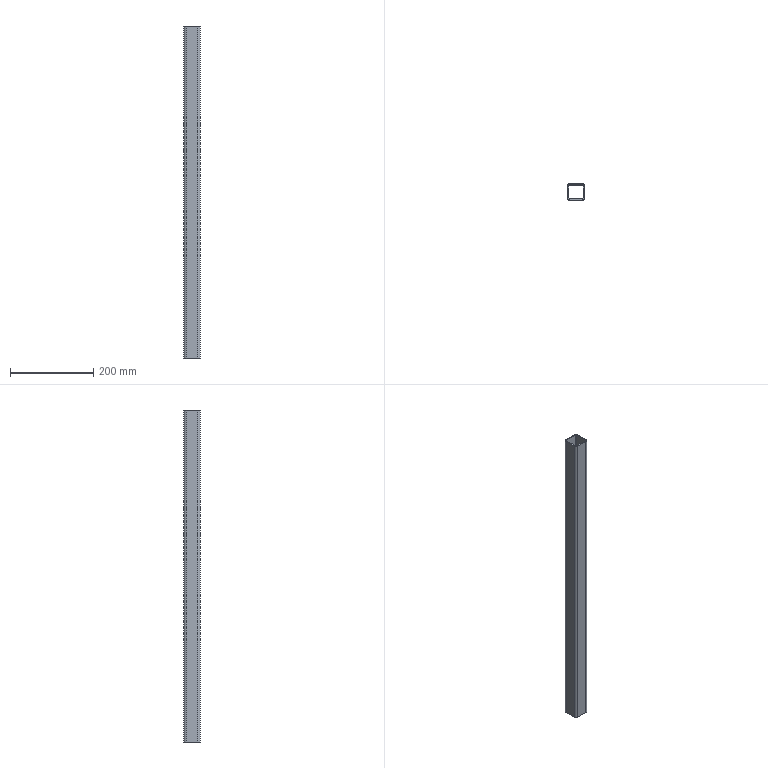Part | STEP file | SN10_002_008-03_TUBO_QUADRADO | 1 solid | 18 faces | box 40 x 40 x 800 mm | volume 336658 mm3 | plane 10 | cylinder 8 | commonest cylinder face diameters 6 x4 12 x4
STEP:
#1=CARTESIAN_POINT('',(0.,0.,0.));
#2=DIRECTION('',(0.,0.,1.));
#3=DIRECTION('',(1.,0.,0.));
#4=AXIS2_PLACEMENT_3D('',#1,#2,#3);
#5=CARTESIAN_POINT('',(20.,14.,-800.));
#6=VERTEX_POINT('',#5);
#7=CARTESIAN_POINT('',(14.,20.,-800.));
#8=VERTEX_POINT('',#7);
#9=CARTESIAN_POINT('',(14.,14.,-800.));
#10=DIRECTION('',(0.,0.,1.));
#11=DIRECTION('',(1.,0.,0.));
#12=AXIS2_PLACEMENT_3D('',#9,#10,#11);
#13=CIRCLE('',#12,6.);
#14=CARTESIAN_POINT('',(14.,14.,-400.));
#15=DIRECTION('',(0.,0.,1.));
#16=DIRECTION('',(1.,0.,0.));
#17=AXIS2_PLACEMENT_3D('',#14,#15,#16);
#18=CYLINDRICAL_SURFACE('',#17,6.);
#19=CARTESIAN_POINT('',(0.,-400.));
#20=DIRECTION('',(1.,0.));
#21=VECTOR('',#20,1.);
#22=LINE('',#19,#21);
#23=(GEOMETRIC_REPRESENTATION_CONTEXT(2)PARAMETRIC_REPRESENTATION_CONTEXT()REPRESENTATION_CONTEXT('',''));
#24=DEFINITIONAL_REPRESENTATION('',(#22),#23);
#25=PCURVE('',#18,#24);
#26=CARTESIAN_POINT('',(0.,0.,-800.));
#27=DIRECTION('',(0.,0.,1.));
#28=DIRECTION('',(1.,0.,0.));
#29=AXIS2_PLACEMENT_3D('',#26,#27,#28);
#30=PLANE('',#29);
#31=CARTESIAN_POINT('',(14.,14.));
#32=DIRECTION('',(1.,0.));
#33=AXIS2_PLACEMENT_2D('',#31,#32);
#34=CIRCLE('',#33,6.);
#35=(GEOMETRIC_REPRESENTATION_CONTEXT(2)PARAMETRIC_REPRESENTATION_CONTEXT()REPRESENTATION_CONTEXT('',''));
#36=DEFINITIONAL_REPRESENTATION('',(#34),#35);
#37=PCURVE('',#30,#36);
#38=SURFACE_CURVE('',#13,(#25,#37),.PCURVE_S1.);
#39=EDGE_CURVE('',#6,#8,#38,.T.);
#40=ORIENTED_EDGE('',*,*,#39,.T.);
#41=CARTESIAN_POINT('',(14.,20.,0.));
#42=VERTEX_POINT('',#41);
#43=CARTESIAN_POINT('',(14.,20.,-800.));
#44=DIRECTION('',(0.,0.,1.));
#45=VECTOR('',#44,1.);
#46=LINE('',#43,#45);
#47=CARTESIAN_POINT('',(1.571,-400.));
#48=DIRECTION('',(0.,1.));
#49=VECTOR('',#48,1.);
#50=LINE('',#47,#49);
#51=(GEOMETRIC_REPRESENTATION_CONTEXT(2)PARAMETRIC_REPRESENTATION_CONTEXT()REPRESENTATION_CONTEXT('',''));
#52=DEFINITIONAL_REPRESENTATION('',(#50),#51);
#53=PCURVE('',#18,#52);
#54=CARTESIAN_POINT('',(-14.,20.,0.));
#55=DIRECTION('',(0.,1.,0.));
#56=DIRECTION('',(0.,0.,1.));
#57=AXIS2_PLACEMENT_3D('',#54,#55,#56);
#58=PLANE('',#57);
#59=CARTESIAN_POINT('',(-800.,28.));
#60=DIRECTION('',(1.,0.));
#61=VECTOR('',#60,1.);
#62=LINE('',#59,#61);
#63=(GEOMETRIC_REPRESENTATION_CONTEXT(2)PARAMETRIC_REPRESENTATION_CONTEXT()REPRESENTATION_CONTEXT('',''));
#64=DEFINITIONAL_REPRESENTATION('',(#62),#63);
#65=PCURVE('',#58,#64);
#66=SURFACE_CURVE('',#46,(#53,#65),.PCURVE_S1.);
#67=EDGE_CURVE('',#8,#42,#66,.T.);
#68=ORIENTED_EDGE('',*,*,#67,.T.);
#69=CARTESIAN_POINT('',(20.,14.,0.));
#70=VERTEX_POINT('',#69);
#71=CARTESIAN_POINT('',(14.,14.,0.));
#72=DIRECTION('',(0.,0.,1.));
#73=DIRECTION('',(1.,0.,0.));
#74=AXIS2_PLACEMENT_3D('',#71,#72,#73);
#75=CIRCLE('',#74,6.);
#76=CARTESIAN_POINT('',(0.,400.));
#77=DIRECTION('',(1.,0.));
#78=VECTOR('',#77,1.);
#79=LINE('',#76,#78);
#80=(GEOMETRIC_REPRESENTATION_CONTEXT(2)PARAMETRIC_REPRESENTATION_CONTEXT()REPRESENTATION_CONTEXT('',''));
#81=DEFINITIONAL_REPRESENTATION('',(#79),#80);
#82=PCURVE('',#18,#81);
#83=CARTESIAN_POINT('',(0.,0.,0.));
#84=DIRECTION('',(0.,0.,1.));
#85=DIRECTION('',(1.,0.,0.));
#86=AXIS2_PLACEMENT_3D('',#83,#84,#85);
#87=PLANE('',#86);
#88=CARTESIAN_POINT('',(14.,14.));
#89=DIRECTION('',(1.,0.));
#90=AXIS2_PLACEMENT_2D('',#88,#89);
#91=CIRCLE('',#90,6.);
#92=(GEOMETRIC_REPRESENTATION_CONTEXT(2)PARAMETRIC_REPRESENTATION_CONTEXT()REPRESENTATION_CONTEXT('',''));
#93=DEFINITIONAL_REPRESENTATION('',(#91),#92);
#94=PCURVE('',#87,#93);
#95=SURFACE_CURVE('',#75,(#82,#94),.PCURVE_S1.);
#96=EDGE_CURVE('',#70,#42,#95,.T.);
#97=ORIENTED_EDGE('',*,*,#96,.F.);
#98=CARTESIAN_POINT('',(20.,14.,-800.));
#99=DIRECTION('',(0.,0.,1.));
#100=VECTOR('',#99,1.);
#101=LINE('',#98,#100);
#102=CARTESIAN_POINT('',(0.,-400.));
#103=DIRECTION('',(0.,1.));
#104=VECTOR('',#103,1.);
#105=LINE('',#102,#104);
#106=(GEOMETRIC_REPRESENTATION_CONTEXT(2)PARAMETRIC_REPRESENTATION_CONTEXT()REPRESENTATION_CONTEXT('',''));
#107=DEFINITIONAL_REPRESENTATION('',(#105),#106);
#108=PCURVE('',#18,#107);
#109=CARTESIAN_POINT('',(20.,14.,0.));
#110=DIRECTION('',(1.,0.,0.));
#111=DIRECTION('',(0.,0.,-1.));
#112=AXIS2_PLACEMENT_3D('',#109,#110,#111);
#113=PLANE('',#112);
#114=CARTESIAN_POINT('',(800.,0.));
#115=DIRECTION('',(-1.,0.));
#116=VECTOR('',#115,1.);
#117=LINE('',#114,#116);
#118=(GEOMETRIC_REPRESENTATION_CONTEXT(2)PARAMETRIC_REPRESENTATION_CONTEXT()REPRESENTATION_CONTEXT('',''));
#119=DEFINITIONAL_REPRESENTATION('',(#117),#118);
#120=PCURVE('',#113,#119);
#121=SURFACE_CURVE('',#101,(#108,#120),.PCURVE_S1.);
#122=EDGE_CURVE('',#6,#70,#121,.T.);
#123=ORIENTED_EDGE('',*,*,#122,.F.);
#124=EDGE_LOOP('',(#40,#68,#97,#123));
#125=FACE_BOUND('',#124,.T.);
#126=ADVANCED_FACE('',(#125),#18,.T.);
#127=CARTESIAN_POINT('',(-14.,20.,-800.));
#128=VERTEX_POINT('',#127);
#129=CARTESIAN_POINT('',(-14.,20.,-800.));
#130=DIRECTION('',(1.,0.,0.));
#131=VECTOR('',#130,1.);
#132=LINE('',#129,#131);
#133=CARTESIAN_POINT('',(-800.,0.));
#134=DIRECTION('',(0.,1.));
#135=VECTOR('',#134,1.);
#136=LINE('',#133,#135);
#137=(GEOMETRIC_REPRESENTATION_CONTEXT(2)PARAMETRIC_REPRESENTATION_CONTEXT()REPRESENTATION_CONTEXT('',''));
#138=DEFINITIONAL_REPRESENTATION('',(#136),#137);
#139=PCURVE('',#58,#138);
#140=CARTESIAN_POINT('',(-14.,20.));
#141=DIRECTION('',(1.,0.));
#142=VECTOR('',#141,1.);
#143=LINE('',#140,#142);
#144=(GEOMETRIC_REPRESENTATION_CONTEXT(2)PARAMETRIC_REPRESENTATION_CONTEXT()REPRESENTATION_CONTEXT('',''));
#145=DEFINITIONAL_REPRESENTATION('',(#143),#144);
#146=PCURVE('',#30,#145);
#147=SURFACE_CURVE('',#132,(#139,#146),.PCURVE_S1.);
#148=EDGE_CURVE('',#128,#8,#147,.T.);
#149=ORIENTED_EDGE('',*,*,#148,.F.);
#150=CARTESIAN_POINT('',(-14.,20.,0.));
#151=VERTEX_POINT('',#150);
#152=CARTESIAN_POINT('',(-14.,20.,0.));
#153=DIRECTION('',(0.,0.,-1.));
#154=VECTOR('',#153,1.);
#155=LINE('',#152,#154);
#156=CARTESIAN_POINT('',(0.,0.));
#157=DIRECTION('',(-1.,0.));
#158=VECTOR('',#157,1.);
#159=LINE('',#156,#158);
#160=(GEOMETRIC_REPRESENTATION_CONTEXT(2)PARAMETRIC_REPRESENTATION_CONTEXT()REPRESENTATION_CONTEXT('',''));
#161=DEFINITIONAL_REPRESENTATION('',(#159),#160);
#162=PCURVE('',#58,#161);
#163=CARTESIAN_POINT('',(-14.,14.,-400.));
#164=DIRECTION('',(0.,0.,1.));
#165=DIRECTION('',(0.,1.,0.));
#166=AXIS2_PLACEMENT_3D('',#163,#164,#165);
#167=CYLINDRICAL_SURFACE('',#166,6.);
#168=CARTESIAN_POINT('',(0.,400.));
#169=DIRECTION('',(0.,-1.));
#170=VECTOR('',#169,1.);
#171=LINE('',#168,#170);
#172=(GEOMETRIC_REPRESENTATION_CONTEXT(2)PARAMETRIC_REPRESENTATION_CONTEXT()REPRESENTATION_CONTEXT('',''));
#173=DEFINITIONAL_REPRESENTATION('',(#171),#172);
#174=PCURVE('',#167,#173);
#175=SURFACE_CURVE('',#155,(#162,#174),.PCURVE_S1.);
#176=EDGE_CURVE('',#151,#128,#175,.T.);
#177=ORIENTED_EDGE('',*,*,#176,.F.);
#178=CARTESIAN_POINT('',(-14.,20.,0.));
#179=DIRECTION('',(1.,0.,0.));
#180=VECTOR('',#179,1.);
#181=LINE('',#178,#180);
#182=CARTESIAN_POINT('',(0.,0.));
#183=DIRECTION('',(0.,1.));
#184=VECTOR('',#183,1.);
#185=LINE('',#182,#184);
#186=(GEOMETRIC_REPRESENTATION_CONTEXT(2)PARAMETRIC_REPRESENTATION_CONTEXT()REPRESENTATION_CONTEXT('',''));
#187=DEFINITIONAL_REPRESENTATION('',(#185),#186);
#188=PCURVE('',#58,#187);
#189=CARTESIAN_POINT('',(-14.,20.));
#190=DIRECTION('',(1.,0.));
#191=VECTOR('',#190,1.);
#192=LINE('',#189,#191);
#193=(GEOMETRIC_REPRESENTATION_CONTEXT(2)PARAMETRIC_REPRESENTATION_CONTEXT()REPRESENTATION_CONTEXT('',''));
#194=DEFINITIONAL_REPRESENTATION('',(#192),#193);
#195=PCURVE('',#87,#194);
#196=SURFACE_CURVE('',#181,(#188,#195),.PCURVE_S1.);
#197=EDGE_CURVE('',#151,#42,#196,.T.);
#198=ORIENTED_EDGE('',*,*,#197,.T.);
#199=ORIENTED_EDGE('',*,*,#67,.F.);
#200=EDGE_LOOP('',(#149,#177,#198,#199));
#201=FACE_BOUND('',#200,.T.);
#202=ADVANCED_FACE('',(#201),#58,.T.);
#203=CARTESIAN_POINT('',(-20.,14.,-800.));
#204=VERTEX_POINT('',#203);
#205=CARTESIAN_POINT('',(-14.,14.,-800.));
#206=DIRECTION('',(0.,0.,1.));
#207=DIRECTION('',(1.,0.,0.));
#208=AXIS2_PLACEMENT_3D('',#205,#206,#207);
#209=CIRCLE('',#208,6.);
#210=CARTESIAN_POINT('',(-1.571,-400.));
#211=DIRECTION('',(1.,0.));
#212=VECTOR('',#211,1.);
#213=LINE('',#210,#212);
#214=(GEOMETRIC_REPRESENTATION_CONTEXT(2)PARAMETRIC_REPRESENTATION_CONTEXT()REPRESENTATION_CONTEXT('',''));
#215=DEFINITIONAL_REPRESENTATION('',(#213),#214);
#216=PCURVE('',#167,#215);
#217=CARTESIAN_POINT('',(-14.,14.));
#218=DIRECTION('',(1.,0.));
#219=AXIS2_PLACEMENT_2D('',#217,#218);
#220=CIRCLE('',#219,6.);
#221=(GEOMETRIC_REPRESENTATION_CONTEXT(2)PARAMETRIC_REPRESENTATION_CONTEXT()REPRESENTATION_CONTEXT('',''));
#222=DEFINITIONAL_REPRESENTATION('',(#220),#221);
#223=PCURVE('',#30,#222);
#224=SURFACE_CURVE('',#209,(#216,#223),.PCURVE_S1.);
#225=EDGE_CURVE('',#128,#204,#224,.T.);
#226=ORIENTED_EDGE('',*,*,#225,.T.);
#227=CARTESIAN_POINT('',(-20.,14.,0.));
#228=VERTEX_POINT('',#227);
#229=CARTESIAN_POINT('',(-20.,14.,-800.));
#230=DIRECTION('',(0.,0.,1.));
#231=VECTOR('',#230,1.);
#232=LINE('',#229,#231);
#233=CARTESIAN_POINT('',(1.571,-400.));
#234=DIRECTION('',(0.,1.));
#235=VECTOR('',#234,1.);
#236=LINE('',#233,#235);
#237=(GEOMETRIC_REPRESENTATION_CONTEXT(2)PARAMETRIC_REPRESENTATION_CONTEXT()REPRESENTATION_CONTEXT('',''));
#238=DEFINITIONAL_REPRESENTATION('',(#236),#237);
#239=PCURVE('',#167,#238);
#240=CARTESIAN_POINT('',(-20.,-14.,0.));
#241=DIRECTION('',(-1.,0.,0.));
#242=DIRECTION('',(0.,0.,1.));
#243=AXIS2_PLACEMENT_3D('',#240,#241,#242);
#244=PLANE('',#243);
#245=CARTESIAN_POINT('',(-800.,28.));
#246=DIRECTION('',(1.,0.));
#247=VECTOR('',#246,1.);
#248=LINE('',#245,#247);
#249=(GEOMETRIC_REPRESENTATION_CONTEXT(2)PARAMETRIC_REPRESENTATION_CONTEXT()REPRESENTATION_CONTEXT('',''));
#250=DEFINITIONAL_REPRESENTATION('',(#248),#249);
#251=PCURVE('',#244,#250);
#252=SURFACE_CURVE('',#232,(#239,#251),.PCURVE_S1.);
#253=EDGE_CURVE('',#204,#228,#252,.T.);
#254=ORIENTED_EDGE('',*,*,#253,.T.);
#255=CARTESIAN_POINT('',(-14.,14.,0.));
#256=DIRECTION('',(0.,0.,1.));
#257=DIRECTION('',(1.,0.,0.));
#258=AXIS2_PLACEMENT_3D('',#255,#256,#257);
#259=CIRCLE('',#258,6.);
#260=CARTESIAN_POINT('',(-1.571,400.));
#261=DIRECTION('',(1.,0.));
#262=VECTOR('',#261,1.);
#263=LINE('',#260,#262);
#264=(GEOMETRIC_REPRESENTATION_CONTEXT(2)PARAMETRIC_REPRESENTATION_CONTEXT()REPRESENTATION_CONTEXT('',''));
#265=DEFINITIONAL_REPRESENTATION('',(#263),#264);
#266=PCURVE('',#167,#265);
#267=CARTESIAN_POINT('',(-14.,14.));
#268=DIRECTION('',(1.,0.));
#269=AXIS2_PLACEMENT_2D('',#267,#268);
#270=CIRCLE('',#269,6.);
#271=(GEOMETRIC_REPRESENTATION_CONTEXT(2)PARAMETRIC_REPRESENTATION_CONTEXT()REPRESENTATION_CONTEXT('',''));
#272=DEFINITIONAL_REPRESENTATION('',(#270),#271);
#273=PCURVE('',#87,#272);
#274=SURFACE_CURVE('',#259,(#266,#273),.PCURVE_S1.);
#275=EDGE_CURVE('',#151,#228,#274,.T.);
#276=ORIENTED_EDGE('',*,*,#275,.F.);
#277=ORIENTED_EDGE('',*,*,#176,.T.);
#278=EDGE_LOOP('',(#226,#254,#276,#277));
#279=FACE_BOUND('',#278,.T.);
#280=ADVANCED_FACE('',(#279),#167,.T.);
#281=CARTESIAN_POINT('',(-20.,-14.,-800.));
#282=VERTEX_POINT('',#281);
#283=CARTESIAN_POINT('',(-20.,-14.,-800.));
#284=DIRECTION('',(0.,1.,0.));
#285=VECTOR('',#284,1.);
#286=LINE('',#283,#285);
#287=CARTESIAN_POINT('',(-800.,0.));
#288=DIRECTION('',(0.,1.));
#289=VECTOR('',#288,1.);
#290=LINE('',#287,#289);
#291=(GEOMETRIC_REPRESENTATION_CONTEXT(2)PARAMETRIC_REPRESENTATION_CONTEXT()REPRESENTATION_CONTEXT('',''));
#292=DEFINITIONAL_REPRESENTATION('',(#290),#291);
#293=PCURVE('',#244,#292);
#294=CARTESIAN_POINT('',(-20.,-14.));
#295=DIRECTION('',(0.,1.));
#296=VECTOR('',#295,1.);
#297=LINE('',#294,#296);
#298=(GEOMETRIC_REPRESENTATION_CONTEXT(2)PARAMETRIC_REPRESENTATION_CONTEXT()REPRESENTATION_CONTEXT('',''));
#299=DEFINITIONAL_REPRESENTATION('',(#297),#298);
#300=PCURVE('',#30,#299);
#301=SURFACE_CURVE('',#286,(#293,#300),.PCURVE_S1.);
#302=EDGE_CURVE('',#282,#204,#301,.T.);
#303=ORIENTED_EDGE('',*,*,#302,.F.);
#304=CARTESIAN_POINT('',(-20.,-14.,0.));
#305=VERTEX_POINT('',#304);
#306=CARTESIAN_POINT('',(-20.,-14.,0.));
#307=DIRECTION('',(0.,0.,-1.));
#308=VECTOR('',#307,1.);
#309=LINE('',#306,#308);
#310=CARTESIAN_POINT('',(0.,0.));
#311=DIRECTION('',(-1.,0.));
#312=VECTOR('',#311,1.);
#313=LINE('',#310,#312);
#314=(GEOMETRIC_REPRESENTATION_CONTEXT(2)PARAMETRIC_REPRESENTATION_CONTEXT()REPRESENTATION_CONTEXT('',''));
#315=DEFINITIONAL_REPRESENTATION('',(#313),#314);
#316=PCURVE('',#244,#315);
#317=CARTESIAN_POINT('',(-14.,-14.,-400.));
#318=DIRECTION('',(0.,0.,1.));
#319=DIRECTION('',(-1.,0.,0.));
#320=AXIS2_PLACEMENT_3D('',#317,#318,#319);
#321=CYLINDRICAL_SURFACE('',#320,6.);
#322=CARTESIAN_POINT('',(0.,400.));
#323=DIRECTION('',(0.,-1.));
#324=VECTOR('',#323,1.);
#325=LINE('',#322,#324);
#326=(GEOMETRIC_REPRESENTATION_CONTEXT(2)PARAMETRIC_REPRESENTATION_CONTEXT()REPRESENTATION_CONTEXT('',''));
#327=DEFINITIONAL_REPRESENTATION('',(#325),#326);
#328=PCURVE('',#321,#327);
#329=SURFACE_CURVE('',#309,(#316,#328),.PCURVE_S1.);
#330=EDGE_CURVE('',#305,#282,#329,.T.);
#331=ORIENTED_EDGE('',*,*,#330,.F.);
#332=CARTESIAN_POINT('',(-20.,-14.,0.));
#333=DIRECTION('',(0.,1.,0.));
#334=VECTOR('',#333,1.);
#335=LINE('',#332,#334);
#336=CARTESIAN_POINT('',(0.,0.));
#337=DIRECTION('',(0.,1.));
#338=VECTOR('',#337,1.);
#339=LINE('',#336,#338);
#340=(GEOMETRIC_REPRESENTATION_CONTEXT(2)PARAMETRIC_REPRESENTATION_CONTEXT()REPRESENTATION_CONTEXT('',''));
#341=DEFINITIONAL_REPRESENTATION('',(#339),#340);
#342=PCURVE('',#244,#341);
#343=CARTESIAN_POINT('',(-20.,-14.));
#344=DIRECTION('',(0.,1.));
#345=VECTOR('',#344,1.);
#346=LINE('',#343,#345);
#347=(GEOMETRIC_REPRESENTATION_CONTEXT(2)PARAMETRIC_REPRESENTATION_CONTEXT()REPRESENTATION_CONTEXT('',''));
#348=DEFINITIONAL_REPRESENTATION('',(#346),#347);
#349=PCURVE('',#87,#348);
#350=SURFACE_CURVE('',#335,(#342,#349),.PCURVE_S1.);
#351=EDGE_CURVE('',#305,#228,#350,.T.);
#352=ORIENTED_EDGE('',*,*,#351,.T.);
#353=ORIENTED_EDGE('',*,*,#253,.F.);
#354=EDGE_LOOP('',(#303,#331,#352,#353));
#355=FACE_BOUND('',#354,.T.);
#356=ADVANCED_FACE('',(#355),#244,.T.);
#357=CARTESIAN_POINT('',(-14.,-20.,-800.));
#358=VERTEX_POINT('',#357);
#359=CARTESIAN_POINT('',(-14.,-14.,-800.));
#360=DIRECTION('',(0.,0.,1.));
#361=DIRECTION('',(1.,0.,0.));
#362=AXIS2_PLACEMENT_3D('',#359,#360,#361);
#363=CIRCLE('',#362,6.);
#364=CARTESIAN_POINT('',(-3.142,-400.));
#365=DIRECTION('',(1.,0.));
#366=VECTOR('',#365,1.);
#367=LINE('',#364,#366);
#368=(GEOMETRIC_REPRESENTATION_CONTEXT(2)PARAMETRIC_REPRESENTATION_CONTEXT()REPRESENTATION_CONTEXT('',''));
#369=DEFINITIONAL_REPRESENTATION('',(#367),#368);
#370=PCURVE('',#321,#369);
#371=CARTESIAN_POINT('',(-14.,-14.));
#372=DIRECTION('',(1.,0.));
#373=AXIS2_PLACEMENT_2D('',#371,#372);
#374=CIRCLE('',#373,6.);
#375=(GEOMETRIC_REPRESENTATION_CONTEXT(2)PARAMETRIC_REPRESENTATION_CONTEXT()REPRESENTATION_CONTEXT('',''));
#376=DEFINITIONAL_REPRESENTATION('',(#374),#375);
#377=PCURVE('',#30,#376);
#378=SURFACE_CURVE('',#363,(#370,#377),.PCURVE_S1.);
#379=EDGE_CURVE('',#282,#358,#378,.T.);
#380=ORIENTED_EDGE('',*,*,#379,.T.);
#381=CARTESIAN_POINT('',(-14.,-20.,0.));
#382=VERTEX_POINT('',#381);
#383=CARTESIAN_POINT('',(-14.,-20.,-800.));
#384=DIRECTION('',(0.,0.,1.));
#385=VECTOR('',#384,1.);
#386=LINE('',#383,#385);
#387=CARTESIAN_POINT('',(1.571,-400.));
#388=DIRECTION('',(0.,1.));
#389=VECTOR('',#388,1.);
#390=LINE('',#387,#389);
#391=(GEOMETRIC_REPRESENTATION_CONTEXT(2)PARAMETRIC_REPRESENTATION_CONTEXT()REPRESENTATION_CONTEXT('',''));
#392=DEFINITIONAL_REPRESENTATION('',(#390),#391);
#393=PCURVE('',#321,#392);
#394=CARTESIAN_POINT('',(14.,-20.,0.));
#395=DIRECTION('',(0.,-1.,0.));
#396=DIRECTION('',(0.,0.,-1.));
#397=AXIS2_PLACEMENT_3D('',#394,#395,#396);
#398=PLANE('',#397);
#399=CARTESIAN_POINT('',(800.,-28.));
#400=DIRECTION('',(-1.,0.));
#401=VECTOR('',#400,1.);
#402=LINE('',#399,#401);
#403=(GEOMETRIC_REPRESENTATION_CONTEXT(2)PARAMETRIC_REPRESENTATION_CONTEXT()REPRESENTATION_CONTEXT('',''));
#404=DEFINITIONAL_REPRESENTATION('',(#402),#403);
#405=PCURVE('',#398,#404);
#406=SURFACE_CURVE('',#386,(#393,#405),.PCURVE_S1.);
#407=EDGE_CURVE('',#358,#382,#406,.T.);
#408=ORIENTED_EDGE('',*,*,#407,.T.);
#409=CARTESIAN_POINT('',(-14.,-14.,0.));
#410=DIRECTION('',(0.,0.,1.));
#411=DIRECTION('',(1.,0.,0.));
#412=AXIS2_PLACEMENT_3D('',#409,#410,#411);
#413=CIRCLE('',#412,6.);
#414=CARTESIAN_POINT('',(-3.142,400.));
#415=DIRECTION('',(1.,0.));
#416=VECTOR('',#415,1.);
#417=LINE('',#414,#416);
#418=(GEOMETRIC_REPRESENTATION_CONTEXT(2)PARAMETRIC_REPRESENTATION_CONTEXT()REPRESENTATION_CONTEXT('',''));
#419=DEFINITIONAL_REPRESENTATION('',(#417),#418);
#420=PCURVE('',#321,#419);
#421=CARTESIAN_POINT('',(-14.,-14.));
#422=DIRECTION('',(1.,0.));
#423=AXIS2_PLACEMENT_2D('',#421,#422);
#424=CIRCLE('',#423,6.);
#425=(GEOMETRIC_REPRESENTATION_CONTEXT(2)PARAMETRIC_REPRESENTATION_CONTEXT()REPRESENTATION_CONTEXT('',''));
#426=DEFINITIONAL_REPRESENTATION('',(#424),#425);
#427=PCURVE('',#87,#426);
#428=SURFACE_CURVE('',#413,(#420,#427),.PCURVE_S1.);
#429=EDGE_CURVE('',#305,#382,#428,.T.);
#430=ORIENTED_EDGE('',*,*,#429,.F.);
#431=ORIENTED_EDGE('',*,*,#330,.T.);
#432=EDGE_LOOP('',(#380,#408,#430,#431));
#433=FACE_BOUND('',#432,.T.);
#434=ADVANCED_FACE('',(#433),#321,.T.);
#435=CARTESIAN_POINT('',(14.,-20.,-800.));
#436=VERTEX_POINT('',#435);
#437=CARTESIAN_POINT('',(14.,-20.,-800.));
#438=DIRECTION('',(-1.,0.,0.));
#439=VECTOR('',#438,1.);
#440=LINE('',#437,#439);
#441=CARTESIAN_POINT('',(800.,0.));
#442=DIRECTION('',(0.,-1.));
#443=VECTOR('',#442,1.);
#444=LINE('',#441,#443);
#445=(GEOMETRIC_REPRESENTATION_CONTEXT(2)PARAMETRIC_REPRESENTATION_CONTEXT()REPRESENTATION_CONTEXT('',''));
#446=DEFINITIONAL_REPRESENTATION('',(#444),#445);
#447=PCURVE('',#398,#446);
#448=CARTESIAN_POINT('',(14.,-20.));
#449=DIRECTION('',(-1.,0.));
#450=VECTOR('',#449,1.);
#451=LINE('',#448,#450);
#452=(GEOMETRIC_REPRESENTATION_CONTEXT(2)PARAMETRIC_REPRESENTATION_CONTEXT()REPRESENTATION_CONTEXT('',''));
#453=DEFINITIONAL_REPRESENTATION('',(#451),#452);
#454=PCURVE('',#30,#453);
#455=SURFACE_CURVE('',#440,(#447,#454),.PCURVE_S1.);
#456=EDGE_CURVE('',#436,#358,#455,.T.);
#457=ORIENTED_EDGE('',*,*,#456,.F.);
#458=CARTESIAN_POINT('',(14.,-20.,0.));
#459=VERTEX_POINT('',#458);
#460=CARTESIAN_POINT('',(14.,-20.,0.));
#461=DIRECTION('',(0.,0.,-1.));
#462=VECTOR('',#461,1.);
#463=LINE('',#460,#462);
#464=CARTESIAN_POINT('',(0.,0.));
#465=DIRECTION('',(1.,0.));
#466=VECTOR('',#465,1.);
#467=LINE('',#464,#466);
#468=(GEOMETRIC_REPRESENTATION_CONTEXT(2)PARAMETRIC_REPRESENTATION_CONTEXT()REPRESENTATION_CONTEXT('',''));
#469=DEFINITIONAL_REPRESENTATION('',(#467),#468);
#470=PCURVE('',#398,#469);
#471=CARTESIAN_POINT('',(14.,-14.,-400.));
#472=DIRECTION('',(0.,0.,1.));
#473=DIRECTION('',(0.,-1.,0.));
#474=AXIS2_PLACEMENT_3D('',#471,#472,#473);
#475=CYLINDRICAL_SURFACE('',#474,6.);
#476=CARTESIAN_POINT('',(0.,400.));
#477=DIRECTION('',(0.,-1.));
#478=VECTOR('',#477,1.);
#479=LINE('',#476,#478);
#480=(GEOMETRIC_REPRESENTATION_CONTEXT(2)PARAMETRIC_REPRESENTATION_CONTEXT()REPRESENTATION_CONTEXT('',''));
#481=DEFINITIONAL_REPRESENTATION('',(#479),#480);
#482=PCURVE('',#475,#481);
#483=SURFACE_CURVE('',#463,(#470,#482),.PCURVE_S1.);
#484=EDGE_CURVE('',#459,#436,#483,.T.);
#485=ORIENTED_EDGE('',*,*,#484,.F.);
#486=CARTESIAN_POINT('',(14.,-20.,0.));
#487=DIRECTION('',(-1.,0.,0.));
#488=VECTOR('',#487,1.);
#489=LINE('',#486,#488);
#490=CARTESIAN_POINT('',(0.,0.));
#491=DIRECTION('',(0.,-1.));
#492=VECTOR('',#491,1.);
#493=LINE('',#490,#492);
#494=(GEOMETRIC_REPRESENTATION_CONTEXT(2)PARAMETRIC_REPRESENTATION_CONTEXT()REPRESENTATION_CONTEXT('',''));
#495=DEFINITIONAL_REPRESENTATION('',(#493),#494);
#496=PCURVE('',#398,#495);
#497=CARTESIAN_POINT('',(14.,-20.));
#498=DIRECTION('',(-1.,0.));
#499=VECTOR('',#498,1.);
#500=LINE('',#497,#499);
#501=(GEOMETRIC_REPRESENTATION_CONTEXT(2)PARAMETRIC_REPRESENTATION_CONTEXT()REPRESENTATION_CONTEXT('',''));
#502=DEFINITIONAL_REPRESENTATION('',(#500),#501);
#503=PCURVE('',#87,#502);
#504=SURFACE_CURVE('',#489,(#496,#503),.PCURVE_S1.);
#505=EDGE_CURVE('',#459,#382,#504,.T.);
#506=ORIENTED_EDGE('',*,*,#505,.T.);
#507=ORIENTED_EDGE('',*,*,#407,.F.);
#508=EDGE_LOOP('',(#457,#485,#506,#507));
#509=FACE_BOUND('',#508,.T.);
#510=ADVANCED_FACE('',(#509),#398,.T.);
#511=CARTESIAN_POINT('',(20.,-14.,-800.));
#512=VERTEX_POINT('',#511);
#513=CARTESIAN_POINT('',(14.,-14.,-800.));
#514=DIRECTION('',(0.,0.,1.));
#515=DIRECTION('',(1.,0.,0.));
#516=AXIS2_PLACEMENT_3D('',#513,#514,#515);
#517=CIRCLE('',#516,6.);
#518=CARTESIAN_POINT('',(-4.712,-400.));
#519=DIRECTION('',(1.,0.));
#520=VECTOR('',#519,1.);
#521=LINE('',#518,#520);
#522=(GEOMETRIC_REPRESENTATION_CONTEXT(2)PARAMETRIC_REPRESENTATION_CONTEXT()REPRESENTATION_CONTEXT('',''));
#523=DEFINITIONAL_REPRESENTATION('',(#521),#522);
#524=PCURVE('',#475,#523);
#525=CARTESIAN_POINT('',(14.,-14.));
#526=DIRECTION('',(1.,0.));
#527=AXIS2_PLACEMENT_2D('',#525,#526);
#528=CIRCLE('',#527,6.);
#529=(GEOMETRIC_REPRESENTATION_CONTEXT(2)PARAMETRIC_REPRESENTATION_CONTEXT()REPRESENTATION_CONTEXT('',''));
#530=DEFINITIONAL_REPRESENTATION('',(#528),#529);
#531=PCURVE('',#30,#530);
#532=SURFACE_CURVE('',#517,(#524,#531),.PCURVE_S1.);
#533=EDGE_CURVE('',#436,#512,#532,.T.);
#534=ORIENTED_EDGE('',*,*,#533,.T.);
#535=CARTESIAN_POINT('',(20.,-14.,0.));
#536=VERTEX_POINT('',#535);
#537=CARTESIAN_POINT('',(20.,-14.,-800.));
#538=DIRECTION('',(0.,0.,1.));
#539=VECTOR('',#538,1.);
#540=LINE('',#537,#539);
#541=CARTESIAN_POINT('',(1.571,-400.));
#542=DIRECTION('',(0.,1.));
#543=VECTOR('',#542,1.);
#544=LINE('',#541,#543);
#545=(GEOMETRIC_REPRESENTATION_CONTEXT(2)PARAMETRIC_REPRESENTATION_CONTEXT()REPRESENTATION_CONTEXT('',''));
#546=DEFINITIONAL_REPRESENTATION('',(#544),#545);
#547=PCURVE('',#475,#546);
#548=CARTESIAN_POINT('',(800.,-28.));
#549=DIRECTION('',(-1.,0.));
#550=VECTOR('',#549,1.);
#551=LINE('',#548,#550);
#552=(GEOMETRIC_REPRESENTATION_CONTEXT(2)PARAMETRIC_REPRESENTATION_CONTEXT()REPRESENTATION_CONTEXT('',''));
#553=DEFINITIONAL_REPRESENTATION('',(#551),#552);
#554=PCURVE('',#113,#553);
#555=SURFACE_CURVE('',#540,(#547,#554),.PCURVE_S1.);
#556=EDGE_CURVE('',#512,#536,#555,.T.);
#557=ORIENTED_EDGE('',*,*,#556,.T.);
#558=CARTESIAN_POINT('',(14.,-14.,0.));
#559=DIRECTION('',(0.,0.,1.));
#560=DIRECTION('',(1.,0.,0.));
#561=AXIS2_PLACEMENT_3D('',#558,#559,#560);
#562=CIRCLE('',#561,6.);
#563=CARTESIAN_POINT('',(-4.712,400.));
#564=DIRECTION('',(1.,0.));
#565=VECTOR('',#564,1.);
#566=LINE('',#563,#565);
#567=(GEOMETRIC_REPRESENTATION_CONTEXT(2)PARAMETRIC_REPRESENTATION_CONTEXT()REPRESENTATION_CONTEXT('',''));
#568=DEFINITIONAL_REPRESENTATION('',(#566),#567);
#569=PCURVE('',#475,#568);
#570=CARTESIAN_POINT('',(14.,-14.));
#571=DIRECTION('',(1.,0.));
#572=AXIS2_PLACEMENT_2D('',#570,#571);
#573=CIRCLE('',#572,6.);
#574=(GEOMETRIC_REPRESENTATION_CONTEXT(2)PARAMETRIC_REPRESENTATION_CONTEXT()REPRESENTATION_CONTEXT('',''));
#575=DEFINITIONAL_REPRESENTATION('',(#573),#574);
#576=PCURVE('',#87,#575);
#577=SURFACE_CURVE('',#562,(#569,#576),.PCURVE_S1.);
#578=EDGE_CURVE('',#459,#536,#577,.T.);
#579=ORIENTED_EDGE('',*,*,#578,.F.);
#580=ORIENTED_EDGE('',*,*,#484,.T.);
#581=EDGE_LOOP('',(#534,#557,#579,#580));
#582=FACE_BOUND('',#581,.T.);
#583=ADVANCED_FACE('',(#582),#475,.T.);
#584=CARTESIAN_POINT('',(20.,14.,-800.));
#585=DIRECTION('',(0.,-1.,0.));
#586=VECTOR('',#585,1.);
#587=LINE('',#584,#586);
#588=CARTESIAN_POINT('',(800.,0.));
#589=DIRECTION('',(0.,-1.));
#590=VECTOR('',#589,1.);
#591=LINE('',#588,#590);
#592=(GEOMETRIC_REPRESENTATION_CONTEXT(2)PARAMETRIC_REPRESENTATION_CONTEXT()REPRESENTATION_CONTEXT('',''));
#593=DEFINITIONAL_REPRESENTATION('',(#591),#592);
#594=PCURVE('',#113,#593);
#595=CARTESIAN_POINT('',(20.,14.));
#596=DIRECTION('',(0.,-1.));
#597=VECTOR('',#596,1.);
#598=LINE('',#595,#597);
#599=(GEOMETRIC_REPRESENTATION_CONTEXT(2)PARAMETRIC_REPRESENTATION_CONTEXT()REPRESENTATION_CONTEXT('',''));
#600=DEFINITIONAL_REPRESENTATION('',(#598),#599);
#601=PCURVE('',#30,#600);
#602=SURFACE_CURVE('',#587,(#594,#601),.PCURVE_S1.);
#603=EDGE_CURVE('',#6,#512,#602,.T.);
#604=ORIENTED_EDGE('',*,*,#603,.F.);
#605=ORIENTED_EDGE('',*,*,#122,.T.);
#606=CARTESIAN_POINT('',(20.,14.,0.));
#607=DIRECTION('',(0.,-1.,0.));
#608=VECTOR('',#607,1.);
#609=LINE('',#606,#608);
#610=CARTESIAN_POINT('',(0.,0.));
#611=DIRECTION('',(0.,-1.));
#612=VECTOR('',#611,1.);
#613=LINE('',#610,#612);
#614=(GEOMETRIC_REPRESENTATION_CONTEXT(2)PARAMETRIC_REPRESENTATION_CONTEXT()REPRESENTATION_CONTEXT('',''));
#615=DEFINITIONAL_REPRESENTATION('',(#613),#614);
#616=PCURVE('',#113,#615);
#617=CARTESIAN_POINT('',(20.,14.));
#618=DIRECTION('',(0.,-1.));
#619=VECTOR('',#618,1.);
#620=LINE('',#617,#619);
#621=(GEOMETRIC_REPRESENTATION_CONTEXT(2)PARAMETRIC_REPRESENTATION_CONTEXT()REPRESENTATION_CONTEXT('',''));
#622=DEFINITIONAL_REPRESENTATION('',(#620),#621);
#623=PCURVE('',#87,#622);
#624=SURFACE_CURVE('',#609,(#616,#623),.PCURVE_S1.);
#625=EDGE_CURVE('',#70,#536,#624,.T.);
#626=ORIENTED_EDGE('',*,*,#625,.T.);
#627=ORIENTED_EDGE('',*,*,#556,.F.);
#628=EDGE_LOOP('',(#604,#605,#626,#627));
#629=FACE_BOUND('',#628,.T.);
#630=ADVANCED_FACE('',(#629),#113,.T.);
#631=CARTESIAN_POINT('',(17.,-14.,0.));
#632=VERTEX_POINT('',#631);
#633=CARTESIAN_POINT('',(17.,-14.,-800.));
#634=VERTEX_POINT('',#633);
#635=CARTESIAN_POINT('',(17.,-14.,0.));
#636=DIRECTION('',(0.,0.,-1.));
#637=VECTOR('',#636,1.);
#638=LINE('',#635,#637);
#639=CARTESIAN_POINT('',(17.,14.,0.));
#640=DIRECTION('',(1.,0.,0.));
#641=DIRECTION('',(0.,0.,-1.));
#642=AXIS2_PLACEMENT_3D('',#639,#640,#641);
#643=PLANE('',#642);
#644=CARTESIAN_POINT('',(0.,-28.));
#645=DIRECTION('',(1.,0.));
#646=VECTOR('',#645,1.);
#647=LINE('',#644,#646);
#648=(GEOMETRIC_REPRESENTATION_CONTEXT(2)PARAMETRIC_REPRESENTATION_CONTEXT()REPRESENTATION_CONTEXT('',''));
#649=DEFINITIONAL_REPRESENTATION('',(#647),#648);
#650=PCURVE('',#643,#649);
#651=CARTESIAN_POINT('',(14.,-14.,-400.));
#652=DIRECTION('',(0.,0.,1.));
#653=DIRECTION('',(0.,-1.,0.));
#654=AXIS2_PLACEMENT_3D('',#651,#652,#653);
#655=CYLINDRICAL_SURFACE('',#654,3.);
#656=CARTESIAN_POINT('',(1.571,400.));
#657=DIRECTION('',(0.,-1.));
#658=VECTOR('',#657,1.);
#659=LINE('',#656,#658);
#660=(GEOMETRIC_REPRESENTATION_CONTEXT(2)PARAMETRIC_REPRESENTATION_CONTEXT()REPRESENTATION_CONTEXT('',''));
#661=DEFINITIONAL_REPRESENTATION('',(#659),#660);
#662=PCURVE('',#655,#661);
#663=SURFACE_CURVE('',#638,(#650,#662),.PCURVE_S1.);
#664=EDGE_CURVE('',#632,#634,#663,.T.);
#665=ORIENTED_EDGE('',*,*,#664,.F.);
#666=CARTESIAN_POINT('',(17.,14.,0.));
#667=VERTEX_POINT('',#666);
#668=CARTESIAN_POINT('',(17.,14.,0.));
#669=DIRECTION('',(0.,-1.,0.));
#670=VECTOR('',#669,1.);
#671=LINE('',#668,#670);
#672=CARTESIAN_POINT('',(0.,0.));
#673=DIRECTION('',(0.,-1.));
#674=VECTOR('',#673,1.);
#675=LINE('',#672,#674);
#676=(GEOMETRIC_REPRESENTATION_CONTEXT(2)PARAMETRIC_REPRESENTATION_CONTEXT()REPRESENTATION_CONTEXT('',''));
#677=DEFINITIONAL_REPRESENTATION('',(#675),#676);
#678=PCURVE('',#643,#677);
#679=CARTESIAN_POINT('',(17.,14.));
#680=DIRECTION('',(0.,-1.));
#681=VECTOR('',#680,1.);
#682=LINE('',#679,#681);
#683=(GEOMETRIC_REPRESENTATION_CONTEXT(2)PARAMETRIC_REPRESENTATION_CONTEXT()REPRESENTATION_CONTEXT('',''));
#684=DEFINITIONAL_REPRESENTATION('',(#682),#683);
#685=PCURVE('',#87,#684);
#686=SURFACE_CURVE('',#671,(#678,#685),.PCURVE_S1.);
#687=EDGE_CURVE('',#667,#632,#686,.T.);
#688=ORIENTED_EDGE('',*,*,#687,.F.);
#689=CARTESIAN_POINT('',(17.,14.,-800.));
#690=VERTEX_POINT('',#689);
#691=CARTESIAN_POINT('',(17.,14.,0.));
#692=DIRECTION('',(0.,0.,-1.));
#693=VECTOR('',#692,1.);
#694=LINE('',#691,#693);
#695=CARTESIAN_POINT('',(0.,0.));
#696=DIRECTION('',(1.,0.));
#697=VECTOR('',#696,1.);
#698=LINE('',#695,#697);
#699=(GEOMETRIC_REPRESENTATION_CONTEXT(2)PARAMETRIC_REPRESENTATION_CONTEXT()REPRESENTATION_CONTEXT('',''));
#700=DEFINITIONAL_REPRESENTATION('',(#698),#699);
#701=PCURVE('',#643,#700);
#702=CARTESIAN_POINT('',(14.,14.,-400.));
#703=DIRECTION('',(0.,0.,1.));
#704=DIRECTION('',(1.,0.,0.));
#705=AXIS2_PLACEMENT_3D('',#702,#703,#704);
#706=CYLINDRICAL_SURFACE('',#705,3.);
#707=CARTESIAN_POINT('',(0.,400.));
#708=DIRECTION('',(0.,-1.));
#709=VECTOR('',#708,1.);
#710=LINE('',#707,#709);
#711=(GEOMETRIC_REPRESENTATION_CONTEXT(2)PARAMETRIC_REPRESENTATION_CONTEXT()REPRESENTATION_CONTEXT('',''));
#712=DEFINITIONAL_REPRESENTATION('',(#710),#711);
#713=PCURVE('',#706,#712);
#714=SURFACE_CURVE('',#694,(#701,#713),.PCURVE_S1.);
#715=EDGE_CURVE('',#667,#690,#714,.T.);
#716=ORIENTED_EDGE('',*,*,#715,.T.);
#717=CARTESIAN_POINT('',(17.,14.,-800.));
#718=DIRECTION('',(0.,-1.,0.));
#719=VECTOR('',#718,1.);
#720=LINE('',#717,#719);
#721=CARTESIAN_POINT('',(800.,0.));
#722=DIRECTION('',(0.,-1.));
#723=VECTOR('',#722,1.);
#724=LINE('',#721,#723);
#725=(GEOMETRIC_REPRESENTATION_CONTEXT(2)PARAMETRIC_REPRESENTATION_CONTEXT()REPRESENTATION_CONTEXT('',''));
#726=DEFINITIONAL_REPRESENTATION('',(#724),#725);
#727=PCURVE('',#643,#726);
#728=CARTESIAN_POINT('',(17.,14.));
#729=DIRECTION('',(0.,-1.));
#730=VECTOR('',#729,1.);
#731=LINE('',#728,#730);
#732=(GEOMETRIC_REPRESENTATION_CONTEXT(2)PARAMETRIC_REPRESENTATION_CONTEXT()REPRESENTATION_CONTEXT('',''));
#733=DEFINITIONAL_REPRESENTATION('',(#731),#732);
#734=PCURVE('',#30,#733);
#735=SURFACE_CURVE('',#720,(#727,#734),.PCURVE_S1.);
#736=EDGE_CURVE('',#690,#634,#735,.T.);
#737=ORIENTED_EDGE('',*,*,#736,.T.);
#738=EDGE_LOOP('',(#665,#688,#716,#737));
#739=FACE_BOUND('',#738,.T.);
#740=ADVANCED_FACE('',(#739),#643,.F.);
#741=CARTESIAN_POINT('',(14.,-17.,-800.));
#742=VERTEX_POINT('',#741);
#743=CARTESIAN_POINT('',(14.,-14.,-800.));
#744=DIRECTION('',(0.,0.,1.));
#745=DIRECTION('',(1.,0.,0.));
#746=AXIS2_PLACEMENT_3D('',#743,#744,#745);
#747=CIRCLE('',#746,3.);
#748=CARTESIAN_POINT('',(-4.712,-400.));
#749=DIRECTION('',(1.,0.));
#750=VECTOR('',#749,1.);
#751=LINE('',#748,#750);
#752=(GEOMETRIC_REPRESENTATION_CONTEXT(2)PARAMETRIC_REPRESENTATION_CONTEXT()REPRESENTATION_CONTEXT('',''));
#753=DEFINITIONAL_REPRESENTATION('',(#751),#752);
#754=PCURVE('',#655,#753);
#755=CARTESIAN_POINT('',(14.,-14.));
#756=DIRECTION('',(1.,0.));
#757=AXIS2_PLACEMENT_2D('',#755,#756);
#758=CIRCLE('',#757,3.);
#759=(GEOMETRIC_REPRESENTATION_CONTEXT(2)PARAMETRIC_REPRESENTATION_CONTEXT()REPRESENTATION_CONTEXT('',''));
#760=DEFINITIONAL_REPRESENTATION('',(#758),#759);
#761=PCURVE('',#30,#760);
#762=SURFACE_CURVE('',#747,(#754,#761),.PCURVE_S1.);
#763=EDGE_CURVE('',#742,#634,#762,.T.);
#764=ORIENTED_EDGE('',*,*,#763,.T.);
#765=ORIENTED_EDGE('',*,*,#664,.F.);
#766=CARTESIAN_POINT('',(14.,-17.,0.));
#767=VERTEX_POINT('',#766);
#768=CARTESIAN_POINT('',(14.,-14.,0.));
#769=DIRECTION('',(0.,0.,1.));
#770=DIRECTION('',(1.,0.,0.));
#771=AXIS2_PLACEMENT_3D('',#768,#769,#770);
#772=CIRCLE('',#771,3.);
#773=CARTESIAN_POINT('',(-4.712,400.));
#774=DIRECTION('',(1.,0.));
#775=VECTOR('',#774,1.);
#776=LINE('',#773,#775);
#777=(GEOMETRIC_REPRESENTATION_CONTEXT(2)PARAMETRIC_REPRESENTATION_CONTEXT()REPRESENTATION_CONTEXT('',''));
#778=DEFINITIONAL_REPRESENTATION('',(#776),#777);
#779=PCURVE('',#655,#778);
#780=CARTESIAN_POINT('',(14.,-14.));
#781=DIRECTION('',(1.,0.));
#782=AXIS2_PLACEMENT_2D('',#780,#781);
#783=CIRCLE('',#782,3.);
#784=(GEOMETRIC_REPRESENTATION_CONTEXT(2)PARAMETRIC_REPRESENTATION_CONTEXT()REPRESENTATION_CONTEXT('',''));
#785=DEFINITIONAL_REPRESENTATION('',(#783),#784);
#786=PCURVE('',#87,#785);
#787=SURFACE_CURVE('',#772,(#779,#786),.PCURVE_S1.);
#788=EDGE_CURVE('',#767,#632,#787,.T.);
#789=ORIENTED_EDGE('',*,*,#788,.F.);
#790=CARTESIAN_POINT('',(14.,-17.,-800.));
#791=DIRECTION('',(0.,0.,1.));
#792=VECTOR('',#791,1.);
#793=LINE('',#790,#792);
#794=CARTESIAN_POINT('',(0.,-400.));
#795=DIRECTION('',(0.,1.));
#796=VECTOR('',#795,1.);
#797=LINE('',#794,#796);
#798=(GEOMETRIC_REPRESENTATION_CONTEXT(2)PARAMETRIC_REPRESENTATION_CONTEXT()REPRESENTATION_CONTEXT('',''));
#799=DEFINITIONAL_REPRESENTATION('',(#797),#798);
#800=PCURVE('',#655,#799);
#801=CARTESIAN_POINT('',(14.,-17.,0.));
#802=DIRECTION('',(0.,-1.,0.));
#803=DIRECTION('',(0.,0.,-1.));
#804=AXIS2_PLACEMENT_3D('',#801,#802,#803);
#805=PLANE('',#804);
#806=CARTESIAN_POINT('',(800.,0.));
#807=DIRECTION('',(-1.,0.));
#808=VECTOR('',#807,1.);
#809=LINE('',#806,#808);
#810=(GEOMETRIC_REPRESENTATION_CONTEXT(2)PARAMETRIC_REPRESENTATION_CONTEXT()REPRESENTATION_CONTEXT('',''));
#811=DEFINITIONAL_REPRESENTATION('',(#809),#810);
#812=PCURVE('',#805,#811);
#813=SURFACE_CURVE('',#793,(#800,#812),.PCURVE_S1.);
#814=EDGE_CURVE('',#742,#767,#813,.T.);
#815=ORIENTED_EDGE('',*,*,#814,.F.);
#816=EDGE_LOOP('',(#764,#765,#789,#815));
#817=FACE_BOUND('',#816,.F.);
#818=ADVANCED_FACE('',(#817),#655,.F.);
#819=CARTESIAN_POINT('',(-14.,-17.,0.));
#820=VERTEX_POINT('',#819);
#821=CARTESIAN_POINT('',(-14.,-17.,-800.));
#822=VERTEX_POINT('',#821);
#823=CARTESIAN_POINT('',(-14.,-17.,0.));
#824=DIRECTION('',(0.,0.,-1.));
#825=VECTOR('',#824,1.);
#826=LINE('',#823,#825);
#827=CARTESIAN_POINT('',(0.,-28.));
#828=DIRECTION('',(1.,0.));
#829=VECTOR('',#828,1.);
#830=LINE('',#827,#829);
#831=(GEOMETRIC_REPRESENTATION_CONTEXT(2)PARAMETRIC_REPRESENTATION_CONTEXT()REPRESENTATION_CONTEXT('',''));
#832=DEFINITIONAL_REPRESENTATION('',(#830),#831);
#833=PCURVE('',#805,#832);
#834=CARTESIAN_POINT('',(-14.,-14.,-400.));
#835=DIRECTION('',(0.,0.,1.));
#836=DIRECTION('',(-1.,0.,0.));
#837=AXIS2_PLACEMENT_3D('',#834,#835,#836);
#838=CYLINDRICAL_SURFACE('',#837,3.);
#839=CARTESIAN_POINT('',(1.571,400.));
#840=DIRECTION('',(0.,-1.));
#841=VECTOR('',#840,1.);
#842=LINE('',#839,#841);
#843=(GEOMETRIC_REPRESENTATION_CONTEXT(2)PARAMETRIC_REPRESENTATION_CONTEXT()REPRESENTATION_CONTEXT('',''));
#844=DEFINITIONAL_REPRESENTATION('',(#842),#843);
#845=PCURVE('',#838,#844);
#846=SURFACE_CURVE('',#826,(#833,#845),.PCURVE_S1.);
#847=EDGE_CURVE('',#820,#822,#846,.T.);
#848=ORIENTED_EDGE('',*,*,#847,.F.);
#849=CARTESIAN_POINT('',(14.,-17.,0.));
#850=DIRECTION('',(-1.,0.,0.));
#851=VECTOR('',#850,1.);
#852=LINE('',#849,#851);
#853=CARTESIAN_POINT('',(0.,0.));
#854=DIRECTION('',(0.,-1.));
#855=VECTOR('',#854,1.);
#856=LINE('',#853,#855);
#857=(GEOMETRIC_REPRESENTATION_CONTEXT(2)PARAMETRIC_REPRESENTATION_CONTEXT()REPRESENTATION_CONTEXT('',''));
#858=DEFINITIONAL_REPRESENTATION('',(#856),#857);
#859=PCURVE('',#805,#858);
#860=CARTESIAN_POINT('',(14.,-17.));
#861=DIRECTION('',(-1.,0.));
#862=VECTOR('',#861,1.);
#863=LINE('',#860,#862);
#864=(GEOMETRIC_REPRESENTATION_CONTEXT(2)PARAMETRIC_REPRESENTATION_CONTEXT()REPRESENTATION_CONTEXT('',''));
#865=DEFINITIONAL_REPRESENTATION('',(#863),#864);
#866=PCURVE('',#87,#865);
#867=SURFACE_CURVE('',#852,(#859,#866),.PCURVE_S1.);
#868=EDGE_CURVE('',#767,#820,#867,.T.);
#869=ORIENTED_EDGE('',*,*,#868,.F.);
#870=ORIENTED_EDGE('',*,*,#814,.F.);
#871=CARTESIAN_POINT('',(14.,-17.,-800.));
#872=DIRECTION('',(-1.,0.,0.));
#873=VECTOR('',#872,1.);
#874=LINE('',#871,#873);
#875=CARTESIAN_POINT('',(800.,0.));
#876=DIRECTION('',(0.,-1.));
#877=VECTOR('',#876,1.);
#878=LINE('',#875,#877);
#879=(GEOMETRIC_REPRESENTATION_CONTEXT(2)PARAMETRIC_REPRESENTATION_CONTEXT()REPRESENTATION_CONTEXT('',''));
#880=DEFINITIONAL_REPRESENTATION('',(#878),#879);
#881=PCURVE('',#805,#880);
#882=CARTESIAN_POINT('',(14.,-17.));
#883=DIRECTION('',(-1.,0.));
#884=VECTOR('',#883,1.);
#885=LINE('',#882,#884);
#886=(GEOMETRIC_REPRESENTATION_CONTEXT(2)PARAMETRIC_REPRESENTATION_CONTEXT()REPRESENTATION_CONTEXT('',''));
#887=DEFINITIONAL_REPRESENTATION('',(#885),#886);
#888=PCURVE('',#30,#887);
#889=SURFACE_CURVE('',#874,(#881,#888),.PCURVE_S1.);
#890=EDGE_CURVE('',#742,#822,#889,.T.);
#891=ORIENTED_EDGE('',*,*,#890,.T.);
#892=EDGE_LOOP('',(#848,#869,#870,#891));
#893=FACE_BOUND('',#892,.T.);
#894=ADVANCED_FACE('',(#893),#805,.F.);
#895=CARTESIAN_POINT('',(-17.,-14.,-800.));
#896=VERTEX_POINT('',#895);
#897=CARTESIAN_POINT('',(-14.,-14.,-800.));
#898=DIRECTION('',(0.,0.,1.));
#899=DIRECTION('',(1.,0.,0.));
#900=AXIS2_PLACEMENT_3D('',#897,#898,#899);
#901=CIRCLE('',#900,3.);
#902=CARTESIAN_POINT('',(-3.142,-400.));
#903=DIRECTION('',(1.,0.));
#904=VECTOR('',#903,1.);
#905=LINE('',#902,#904);
#906=(GEOMETRIC_REPRESENTATION_CONTEXT(2)PARAMETRIC_REPRESENTATION_CONTEXT()REPRESENTATION_CONTEXT('',''));
#907=DEFINITIONAL_REPRESENTATION('',(#905),#906);
#908=PCURVE('',#838,#907);
#909=CARTESIAN_POINT('',(-14.,-14.));
#910=DIRECTION('',(1.,0.));
#911=AXIS2_PLACEMENT_2D('',#909,#910);
#912=CIRCLE('',#911,3.);
#913=(GEOMETRIC_REPRESENTATION_CONTEXT(2)PARAMETRIC_REPRESENTATION_CONTEXT()REPRESENTATION_CONTEXT('',''));
#914=DEFINITIONAL_REPRESENTATION('',(#912),#913);
#915=PCURVE('',#30,#914);
#916=SURFACE_CURVE('',#901,(#908,#915),.PCURVE_S1.);
#917=EDGE_CURVE('',#896,#822,#916,.T.);
#918=ORIENTED_EDGE('',*,*,#917,.T.);
#919=ORIENTED_EDGE('',*,*,#847,.F.);
#920=CARTESIAN_POINT('',(-17.,-14.,0.));
#921=VERTEX_POINT('',#920);
#922=CARTESIAN_POINT('',(-14.,-14.,0.));
#923=DIRECTION('',(0.,0.,1.));
#924=DIRECTION('',(1.,0.,0.));
#925=AXIS2_PLACEMENT_3D('',#922,#923,#924);
#926=CIRCLE('',#925,3.);
#927=CARTESIAN_POINT('',(-3.142,400.));
#928=DIRECTION('',(1.,0.));
#929=VECTOR('',#928,1.);
#930=LINE('',#927,#929);
#931=(GEOMETRIC_REPRESENTATION_CONTEXT(2)PARAMETRIC_REPRESENTATION_CONTEXT()REPRESENTATION_CONTEXT('',''));
#932=DEFINITIONAL_REPRESENTATION('',(#930),#931);
#933=PCURVE('',#838,#932);
#934=CARTESIAN_POINT('',(-14.,-14.));
#935=DIRECTION('',(1.,0.));
#936=AXIS2_PLACEMENT_2D('',#934,#935);
#937=CIRCLE('',#936,3.);
#938=(GEOMETRIC_REPRESENTATION_CONTEXT(2)PARAMETRIC_REPRESENTATION_CONTEXT()REPRESENTATION_CONTEXT('',''));
#939=DEFINITIONAL_REPRESENTATION('',(#937),#938);
#940=PCURVE('',#87,#939);
#941=SURFACE_CURVE('',#926,(#933,#940),.PCURVE_S1.);
#942=EDGE_CURVE('',#921,#820,#941,.T.);
#943=ORIENTED_EDGE('',*,*,#942,.F.);
#944=CARTESIAN_POINT('',(-17.,-14.,-800.));
#945=DIRECTION('',(0.,0.,1.));
#946=VECTOR('',#945,1.);
#947=LINE('',#944,#946);
#948=CARTESIAN_POINT('',(0.,-400.));
#949=DIRECTION('',(0.,1.));
#950=VECTOR('',#949,1.);
#951=LINE('',#948,#950);
#952=(GEOMETRIC_REPRESENTATION_CONTEXT(2)PARAMETRIC_REPRESENTATION_CONTEXT()REPRESENTATION_CONTEXT('',''));
#953=DEFINITIONAL_REPRESENTATION('',(#951),#952);
#954=PCURVE('',#838,#953);
#955=CARTESIAN_POINT('',(-17.,-14.,0.));
#956=DIRECTION('',(-1.,0.,0.));
#957=DIRECTION('',(0.,0.,1.));
#958=AXIS2_PLACEMENT_3D('',#955,#956,#957);
#959=PLANE('',#958);
#960=CARTESIAN_POINT('',(-800.,0.));
#961=DIRECTION('',(1.,0.));
#962=VECTOR('',#961,1.);
#963=LINE('',#960,#962);
#964=(GEOMETRIC_REPRESENTATION_CONTEXT(2)PARAMETRIC_REPRESENTATION_CONTEXT()REPRESENTATION_CONTEXT('',''));
#965=DEFINITIONAL_REPRESENTATION('',(#963),#964);
#966=PCURVE('',#959,#965);
#967=SURFACE_CURVE('',#947,(#954,#966),.PCURVE_S1.);
#968=EDGE_CURVE('',#896,#921,#967,.T.);
#969=ORIENTED_EDGE('',*,*,#968,.F.);
#970=EDGE_LOOP('',(#918,#919,#943,#969));
#971=FACE_BOUND('',#970,.F.);
#972=ADVANCED_FACE('',(#971),#838,.F.);
#973=CARTESIAN_POINT('',(-17.,14.,0.));
#974=VERTEX_POINT('',#973);
#975=CARTESIAN_POINT('',(-17.,14.,-800.));
#976=VERTEX_POINT('',#975);
#977=CARTESIAN_POINT('',(-17.,14.,0.));
#978=DIRECTION('',(0.,0.,-1.));
#979=VECTOR('',#978,1.);
#980=LINE('',#977,#979);
#981=CARTESIAN_POINT('',(0.,28.));
#982=DIRECTION('',(-1.,0.));
#983=VECTOR('',#982,1.);
#984=LINE('',#981,#983);
#985=(GEOMETRIC_REPRESENTATION_CONTEXT(2)PARAMETRIC_REPRESENTATION_CONTEXT()REPRESENTATION_CONTEXT('',''));
#986=DEFINITIONAL_REPRESENTATION('',(#984),#985);
#987=PCURVE('',#959,#986);
#988=CARTESIAN_POINT('',(-14.,14.,-400.));
#989=DIRECTION('',(0.,0.,1.));
#990=DIRECTION('',(0.,1.,0.));
#991=AXIS2_PLACEMENT_3D('',#988,#989,#990);
#992=CYLINDRICAL_SURFACE('',#991,3.);
#993=CARTESIAN_POINT('',(1.571,400.));
#994=DIRECTION('',(0.,-1.));
#995=VECTOR('',#994,1.);
#996=LINE('',#993,#995);
#997=(GEOMETRIC_REPRESENTATION_CONTEXT(2)PARAMETRIC_REPRESENTATION_CONTEXT()REPRESENTATION_CONTEXT('',''));
#998=DEFINITIONAL_REPRESENTATION('',(#996),#997);
#999=PCURVE('',#992,#998);
#1000=SURFACE_CURVE('',#980,(#987,#999),.PCURVE_S1.);
#1001=EDGE_CURVE('',#974,#976,#1000,.T.);
#1002=ORIENTED_EDGE('',*,*,#1001,.F.);
#1003=CARTESIAN_POINT('',(-17.,-14.,0.));
#1004=DIRECTION('',(0.,1.,0.));
#1005=VECTOR('',#1004,1.);
#1006=LINE('',#1003,#1005);
#1007=CARTESIAN_POINT('',(0.,0.));
#1008=DIRECTION('',(0.,1.));
#1009=VECTOR('',#1008,1.);
#1010=LINE('',#1007,#1009);
#1011=(GEOMETRIC_REPRESENTATION_CONTEXT(2)PARAMETRIC_REPRESENTATION_CONTEXT()REPRESENTATION_CONTEXT('',''));
#1012=DEFINITIONAL_REPRESENTATION('',(#1010),#1011);
#1013=PCURVE('',#959,#1012);
#1014=CARTESIAN_POINT('',(-17.,-14.));
#1015=DIRECTION('',(0.,1.));
#1016=VECTOR('',#1015,1.);
#1017=LINE('',#1014,#1016);
#1018=(GEOMETRIC_REPRESENTATION_CONTEXT(2)PARAMETRIC_REPRESENTATION_CONTEXT()REPRESENTATION_CONTEXT('',''));
#1019=DEFINITIONAL_REPRESENTATION('',(#1017),#1018);
#1020=PCURVE('',#87,#1019);
#1021=SURFACE_CURVE('',#1006,(#1013,#1020),.PCURVE_S1.);
#1022=EDGE_CURVE('',#921,#974,#1021,.T.);
#1023=ORIENTED_EDGE('',*,*,#1022,.F.);
#1024=ORIENTED_EDGE('',*,*,#968,.F.);
#1025=CARTESIAN_POINT('',(-17.,-14.,-800.));
#1026=DIRECTION('',(0.,1.,0.));
#1027=VECTOR('',#1026,1.);
#1028=LINE('',#1025,#1027);
#1029=CARTESIAN_POINT('',(-800.,0.));
#1030=DIRECTION('',(0.,1.));
#1031=VECTOR('',#1030,1.);
#1032=LINE('',#1029,#1031);
#1033=(GEOMETRIC_REPRESENTATION_CONTEXT(2)PARAMETRIC_REPRESENTATION_CONTEXT()REPRESENTATION_CONTEXT('',''));
#1034=DEFINITIONAL_REPRESENTATION('',(#1032),#1033);
#1035=PCURVE('',#959,#1034);
#1036=CARTESIAN_POINT('',(-17.,-14.));
#1037=DIRECTION('',(0.,1.));
#1038=VECTOR('',#1037,1.);
#1039=LINE('',#1036,#1038);
#1040=(GEOMETRIC_REPRESENTATION_CONTEXT(2)PARAMETRIC_REPRESENTATION_CONTEXT()REPRESENTATION_CONTEXT('',''));
#1041=DEFINITIONAL_REPRESENTATION('',(#1039),#1040);
#1042=PCURVE('',#30,#1041);
#1043=SURFACE_CURVE('',#1028,(#1035,#1042),.PCURVE_S1.);
#1044=EDGE_CURVE('',#896,#976,#1043,.T.);
#1045=ORIENTED_EDGE('',*,*,#1044,.T.);
#1046=EDGE_LOOP('',(#1002,#1023,#1024,#1045));
#1047=FACE_BOUND('',#1046,.T.);
#1048=ADVANCED_FACE('',(#1047),#959,.F.);
#1049=CARTESIAN_POINT('',(-14.,17.,-800.));
#1050=VERTEX_POINT('',#1049);
#1051=CARTESIAN_POINT('',(-14.,14.,-800.));
#1052=DIRECTION('',(0.,0.,1.));
#1053=DIRECTION('',(1.,0.,0.));
#1054=AXIS2_PLACEMENT_3D('',#1051,#1052,#1053);
#1055=CIRCLE('',#1054,3.);
#1056=CARTESIAN_POINT('',(-1.571,-400.));
#1057=DIRECTION('',(1.,0.));
#1058=VECTOR('',#1057,1.);
#1059=LINE('',#1056,#1058);
#1060=(GEOMETRIC_REPRESENTATION_CONTEXT(2)PARAMETRIC_REPRESENTATION_CONTEXT()REPRESENTATION_CONTEXT('',''));
#1061=DEFINITIONAL_REPRESENTATION('',(#1059),#1060);
#1062=PCURVE('',#992,#1061);
#1063=CARTESIAN_POINT('',(-14.,14.));
#1064=DIRECTION('',(1.,0.));
#1065=AXIS2_PLACEMENT_2D('',#1063,#1064);
#1066=CIRCLE('',#1065,3.);
#1067=(GEOMETRIC_REPRESENTATION_CONTEXT(2)PARAMETRIC_REPRESENTATION_CONTEXT()REPRESENTATION_CONTEXT('',''));
#1068=DEFINITIONAL_REPRESENTATION('',(#1066),#1067);
#1069=PCURVE('',#30,#1068);
#1070=SURFACE_CURVE('',#1055,(#1062,#1069),.PCURVE_S1.);
#1071=EDGE_CURVE('',#1050,#976,#1070,.T.);
#1072=ORIENTED_EDGE('',*,*,#1071,.T.);
#1073=ORIENTED_EDGE('',*,*,#1001,.F.);
#1074=CARTESIAN_POINT('',(-14.,17.,0.));
#1075=VERTEX_POINT('',#1074);
#1076=CARTESIAN_POINT('',(-14.,14.,0.));
#1077=DIRECTION('',(0.,0.,1.));
#1078=DIRECTION('',(1.,0.,0.));
#1079=AXIS2_PLACEMENT_3D('',#1076,#1077,#1078);
#1080=CIRCLE('',#1079,3.);
#1081=CARTESIAN_POINT('',(-1.571,400.));
#1082=DIRECTION('',(1.,0.));
#1083=VECTOR('',#1082,1.);
#1084=LINE('',#1081,#1083);
#1085=(GEOMETRIC_REPRESENTATION_CONTEXT(2)PARAMETRIC_REPRESENTATION_CONTEXT()REPRESENTATION_CONTEXT('',''));
#1086=DEFINITIONAL_REPRESENTATION('',(#1084),#1085);
#1087=PCURVE('',#992,#1086);
#1088=CARTESIAN_POINT('',(-14.,14.));
#1089=DIRECTION('',(1.,0.));
#1090=AXIS2_PLACEMENT_2D('',#1088,#1089);
#1091=CIRCLE('',#1090,3.);
#1092=(GEOMETRIC_REPRESENTATION_CONTEXT(2)PARAMETRIC_REPRESENTATION_CONTEXT()REPRESENTATION_CONTEXT('',''));
#1093=DEFINITIONAL_REPRESENTATION('',(#1091),#1092);
#1094=PCURVE('',#87,#1093);
#1095=SURFACE_CURVE('',#1080,(#1087,#1094),.PCURVE_S1.);
#1096=EDGE_CURVE('',#1075,#974,#1095,.T.);
#1097=ORIENTED_EDGE('',*,*,#1096,.F.);
#1098=CARTESIAN_POINT('',(-14.,17.,-800.));
#1099=DIRECTION('',(0.,0.,1.));
#1100=VECTOR('',#1099,1.);
#1101=LINE('',#1098,#1100);
#1102=CARTESIAN_POINT('',(0.,-400.));
#1103=DIRECTION('',(0.,1.));
#1104=VECTOR('',#1103,1.);
#1105=LINE('',#1102,#1104);
#1106=(GEOMETRIC_REPRESENTATION_CONTEXT(2)PARAMETRIC_REPRESENTATION_CONTEXT()REPRESENTATION_CONTEXT('',''));
#1107=DEFINITIONAL_REPRESENTATION('',(#1105),#1106);
#1108=PCURVE('',#992,#1107);
#1109=CARTESIAN_POINT('',(-14.,17.,0.));
#1110=DIRECTION('',(0.,1.,0.));
#1111=DIRECTION('',(0.,0.,1.));
#1112=AXIS2_PLACEMENT_3D('',#1109,#1110,#1111);
#1113=PLANE('',#1112);
#1114=CARTESIAN_POINT('',(-800.,0.));
#1115=DIRECTION('',(1.,0.));
#1116=VECTOR('',#1115,1.);
#1117=LINE('',#1114,#1116);
#1118=(GEOMETRIC_REPRESENTATION_CONTEXT(2)PARAMETRIC_REPRESENTATION_CONTEXT()REPRESENTATION_CONTEXT('',''));
#1119=DEFINITIONAL_REPRESENTATION('',(#1117),#1118);
#1120=PCURVE('',#1113,#1119);
#1121=SURFACE_CURVE('',#1101,(#1108,#1120),.PCURVE_S1.);
#1122=EDGE_CURVE('',#1050,#1075,#1121,.T.);
#1123=ORIENTED_EDGE('',*,*,#1122,.F.);
#1124=EDGE_LOOP('',(#1072,#1073,#1097,#1123));
#1125=FACE_BOUND('',#1124,.F.);
#1126=ADVANCED_FACE('',(#1125),#992,.F.);
#1127=CARTESIAN_POINT('',(14.,17.,0.));
#1128=VERTEX_POINT('',#1127);
#1129=CARTESIAN_POINT('',(14.,17.,-800.));
#1130=VERTEX_POINT('',#1129);
#1131=CARTESIAN_POINT('',(14.,17.,0.));
#1132=DIRECTION('',(0.,0.,-1.));
#1133=VECTOR('',#1132,1.);
#1134=LINE('',#1131,#1133);
#1135=CARTESIAN_POINT('',(0.,28.));
#1136=DIRECTION('',(-1.,0.));
#1137=VECTOR('',#1136,1.);
#1138=LINE('',#1135,#1137);
#1139=(GEOMETRIC_REPRESENTATION_CONTEXT(2)PARAMETRIC_REPRESENTATION_CONTEXT()REPRESENTATION_CONTEXT('',''));
#1140=DEFINITIONAL_REPRESENTATION('',(#1138),#1139);
#1141=PCURVE('',#1113,#1140);
#1142=CARTESIAN_POINT('',(1.571,400.));
#1143=DIRECTION('',(0.,-1.));
#1144=VECTOR('',#1143,1.);
#1145=LINE('',#1142,#1144);
#1146=(GEOMETRIC_REPRESENTATION_CONTEXT(2)PARAMETRIC_REPRESENTATION_CONTEXT()REPRESENTATION_CONTEXT('',''));
#1147=DEFINITIONAL_REPRESENTATION('',(#1145),#1146);
#1148=PCURVE('',#706,#1147);
#1149=SURFACE_CURVE('',#1134,(#1141,#1148),.PCURVE_S1.);
#1150=EDGE_CURVE('',#1128,#1130,#1149,.T.);
#1151=ORIENTED_EDGE('',*,*,#1150,.F.);
#1152=CARTESIAN_POINT('',(-14.,17.,0.));
#1153=DIRECTION('',(1.,0.,0.));
#1154=VECTOR('',#1153,1.);
#1155=LINE('',#1152,#1154);
#1156=CARTESIAN_POINT('',(0.,0.));
#1157=DIRECTION('',(0.,1.));
#1158=VECTOR('',#1157,1.);
#1159=LINE('',#1156,#1158);
#1160=(GEOMETRIC_REPRESENTATION_CONTEXT(2)PARAMETRIC_REPRESENTATION_CONTEXT()REPRESENTATION_CONTEXT('',''));
#1161=DEFINITIONAL_REPRESENTATION('',(#1159),#1160);
#1162=PCURVE('',#1113,#1161);
#1163=CARTESIAN_POINT('',(-14.,17.));
#1164=DIRECTION('',(1.,0.));
#1165=VECTOR('',#1164,1.);
#1166=LINE('',#1163,#1165);
#1167=(GEOMETRIC_REPRESENTATION_CONTEXT(2)PARAMETRIC_REPRESENTATION_CONTEXT()REPRESENTATION_CONTEXT('',''));
#1168=DEFINITIONAL_REPRESENTATION('',(#1166),#1167);
#1169=PCURVE('',#87,#1168);
#1170=SURFACE_CURVE('',#1155,(#1162,#1169),.PCURVE_S1.);
#1171=EDGE_CURVE('',#1075,#1128,#1170,.T.);
#1172=ORIENTED_EDGE('',*,*,#1171,.F.);
#1173=ORIENTED_EDGE('',*,*,#1122,.F.);
#1174=CARTESIAN_POINT('',(-14.,17.,-800.));
#1175=DIRECTION('',(1.,0.,0.));
#1176=VECTOR('',#1175,1.);
#1177=LINE('',#1174,#1176);
#1178=CARTESIAN_POINT('',(-800.,0.));
#1179=DIRECTION('',(0.,1.));
#1180=VECTOR('',#1179,1.);
#1181=LINE('',#1178,#1180);
#1182=(GEOMETRIC_REPRESENTATION_CONTEXT(2)PARAMETRIC_REPRESENTATION_CONTEXT()REPRESENTATION_CONTEXT('',''));
#1183=DEFINITIONAL_REPRESENTATION('',(#1181),#1182);
#1184=PCURVE('',#1113,#1183);
#1185=CARTESIAN_POINT('',(-14.,17.));
#1186=DIRECTION('',(1.,0.));
#1187=VECTOR('',#1186,1.);
#1188=LINE('',#1185,#1187);
#1189=(GEOMETRIC_REPRESENTATION_CONTEXT(2)PARAMETRIC_REPRESENTATION_CONTEXT()REPRESENTATION_CONTEXT('',''));
#1190=DEFINITIONAL_REPRESENTATION('',(#1188),#1189);
#1191=PCURVE('',#30,#1190);
#1192=SURFACE_CURVE('',#1177,(#1184,#1191),.PCURVE_S1.);
#1193=EDGE_CURVE('',#1050,#1130,#1192,.T.);
#1194=ORIENTED_EDGE('',*,*,#1193,.T.);
#1195=EDGE_LOOP('',(#1151,#1172,#1173,#1194));
#1196=FACE_BOUND('',#1195,.T.);
#1197=ADVANCED_FACE('',(#1196),#1113,.F.);
#1198=CARTESIAN_POINT('',(14.,14.,-800.));
#1199=DIRECTION('',(0.,0.,1.));
#1200=DIRECTION('',(1.,0.,0.));
#1201=AXIS2_PLACEMENT_3D('',#1198,#1199,#1200);
#1202=CIRCLE('',#1201,3.);
#1203=CARTESIAN_POINT('',(0.,-400.));
#1204=DIRECTION('',(1.,0.));
#1205=VECTOR('',#1204,1.);
#1206=LINE('',#1203,#1205);
#1207=(GEOMETRIC_REPRESENTATION_CONTEXT(2)PARAMETRIC_REPRESENTATION_CONTEXT()REPRESENTATION_CONTEXT('',''));
#1208=DEFINITIONAL_REPRESENTATION('',(#1206),#1207);
#1209=PCURVE('',#706,#1208);
#1210=CARTESIAN_POINT('',(14.,14.));
#1211=DIRECTION('',(1.,0.));
#1212=AXIS2_PLACEMENT_2D('',#1210,#1211);
#1213=CIRCLE('',#1212,3.);
#1214=(GEOMETRIC_REPRESENTATION_CONTEXT(2)PARAMETRIC_REPRESENTATION_CONTEXT()REPRESENTATION_CONTEXT('',''));
#1215=DEFINITIONAL_REPRESENTATION('',(#1213),#1214);
#1216=PCURVE('',#30,#1215);
#1217=SURFACE_CURVE('',#1202,(#1209,#1216),.PCURVE_S1.);
#1218=EDGE_CURVE('',#690,#1130,#1217,.T.);
#1219=ORIENTED_EDGE('',*,*,#1218,.T.);
#1220=ORIENTED_EDGE('',*,*,#1150,.F.);
#1221=CARTESIAN_POINT('',(14.,14.,0.));
#1222=DIRECTION('',(0.,0.,1.));
#1223=DIRECTION('',(1.,0.,0.));
#1224=AXIS2_PLACEMENT_3D('',#1221,#1222,#1223);
#1225=CIRCLE('',#1224,3.);
#1226=CARTESIAN_POINT('',(0.,400.));
#1227=DIRECTION('',(1.,0.));
#1228=VECTOR('',#1227,1.);
#1229=LINE('',#1226,#1228);
#1230=(GEOMETRIC_REPRESENTATION_CONTEXT(2)PARAMETRIC_REPRESENTATION_CONTEXT()REPRESENTATION_CONTEXT('',''));
#1231=DEFINITIONAL_REPRESENTATION('',(#1229),#1230);
#1232=PCURVE('',#706,#1231);
#1233=CARTESIAN_POINT('',(14.,14.));
#1234=DIRECTION('',(1.,0.));
#1235=AXIS2_PLACEMENT_2D('',#1233,#1234);
#1236=CIRCLE('',#1235,3.);
#1237=(GEOMETRIC_REPRESENTATION_CONTEXT(2)PARAMETRIC_REPRESENTATION_CONTEXT()REPRESENTATION_CONTEXT('',''));
#1238=DEFINITIONAL_REPRESENTATION('',(#1236),#1237);
#1239=PCURVE('',#87,#1238);
#1240=SURFACE_CURVE('',#1225,(#1232,#1239),.PCURVE_S1.);
#1241=EDGE_CURVE('',#667,#1128,#1240,.T.);
#1242=ORIENTED_EDGE('',*,*,#1241,.F.);
#1243=ORIENTED_EDGE('',*,*,#715,.T.);
#1244=EDGE_LOOP('',(#1219,#1220,#1242,#1243));
#1245=FACE_BOUND('',#1244,.F.);
#1246=ADVANCED_FACE('',(#1245),#706,.F.);
#1247=ORIENTED_EDGE('',*,*,#96,.T.);
#1248=ORIENTED_EDGE('',*,*,#197,.F.);
#1249=ORIENTED_EDGE('',*,*,#275,.T.);
#1250=ORIENTED_EDGE('',*,*,#351,.F.);
#1251=ORIENTED_EDGE('',*,*,#429,.T.);
#1252=ORIENTED_EDGE('',*,*,#505,.F.);
#1253=ORIENTED_EDGE('',*,*,#578,.T.);
#1254=ORIENTED_EDGE('',*,*,#625,.F.);
#1255=EDGE_LOOP('',(#1247,#1248,#1249,#1250,#1251,#1252,#1253,#1254));
#1256=FACE_BOUND('',#1255,.T.);
#1257=ORIENTED_EDGE('',*,*,#687,.T.);
#1258=ORIENTED_EDGE('',*,*,#788,.F.);
#1259=ORIENTED_EDGE('',*,*,#868,.T.);
#1260=ORIENTED_EDGE('',*,*,#942,.F.);
#1261=ORIENTED_EDGE('',*,*,#1022,.T.);
#1262=ORIENTED_EDGE('',*,*,#1096,.F.);
#1263=ORIENTED_EDGE('',*,*,#1171,.T.);
#1264=ORIENTED_EDGE('',*,*,#1241,.F.);
#1265=EDGE_LOOP('',(#1257,#1258,#1259,#1260,#1261,#1262,#1263,#1264));
#1266=FACE_BOUND('',#1265,.T.);
#1267=ADVANCED_FACE('',(#1256,#1266),#87,.T.);
#1268=ORIENTED_EDGE('',*,*,#603,.T.);
#1269=ORIENTED_EDGE('',*,*,#533,.F.);
#1270=ORIENTED_EDGE('',*,*,#456,.T.);
#1271=ORIENTED_EDGE('',*,*,#379,.F.);
#1272=ORIENTED_EDGE('',*,*,#302,.T.);
#1273=ORIENTED_EDGE('',*,*,#225,.F.);
#1274=ORIENTED_EDGE('',*,*,#148,.T.);
#1275=ORIENTED_EDGE('',*,*,#39,.F.);
#1276=EDGE_LOOP('',(#1268,#1269,#1270,#1271,#1272,#1273,#1274,#1275));
#1277=FACE_BOUND('',#1276,.T.);
#1278=ORIENTED_EDGE('',*,*,#1218,.T.);
#1279=ORIENTED_EDGE('',*,*,#1193,.F.);
#1280=ORIENTED_EDGE('',*,*,#1071,.T.);
#1281=ORIENTED_EDGE('',*,*,#1044,.F.);
#1282=ORIENTED_EDGE('',*,*,#917,.T.);
#1283=ORIENTED_EDGE('',*,*,#890,.F.);
#1284=ORIENTED_EDGE('',*,*,#763,.T.);
#1285=ORIENTED_EDGE('',*,*,#736,.F.);
#1286=EDGE_LOOP('',(#1278,#1279,#1280,#1281,#1282,#1283,#1284,#1285));
#1287=FACE_BOUND('',#1286,.T.);
#1288=ADVANCED_FACE('',(#1277,#1287),#30,.F.);
#1289=CLOSED_SHELL('',(#126,#202,#280,#356,#434,#510,#583,#630,#740,#818,#894,#972,#1048,#1126,#1197,#1246,#1267,#1288));
#1290=MANIFOLD_SOLID_BREP('',#1289);
#1291=(LENGTH_UNIT()NAMED_UNIT(*)SI_UNIT(.MILLI.,.METRE.));
#1292=UNCERTAINTY_MEASURE_WITH_UNIT(LENGTH_MEASURE(0.0000001),#1291,'','');
#1293=(NAMED_UNIT(*)PLANE_ANGLE_UNIT()SI_UNIT($,.RADIAN.));
#1294=(NAMED_UNIT(*)SI_UNIT($,.STERADIAN.)SOLID_ANGLE_UNIT());
#1295=(GEOMETRIC_REPRESENTATION_CONTEXT(3)GLOBAL_UNCERTAINTY_ASSIGNED_CONTEXT((#1292))GLOBAL_UNIT_ASSIGNED_CONTEXT((#1291,#1293,#1294))REPRESENTATION_CONTEXT('',''));
#1296=ADVANCED_BREP_SHAPE_REPRESENTATION('',(#4,#1290),#1295);